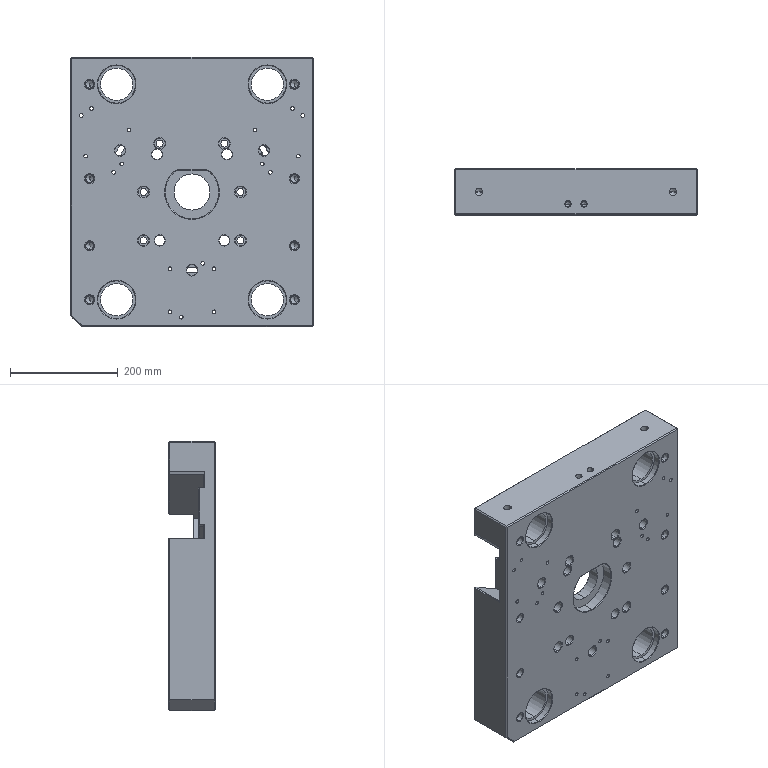Part | STEP file | P2 - 1 cav | 1 solid | 450 faces | box 450 x 86 x 500 mm | volume 13008282 mm3 | cylinder 164 | plane 153 | cone 133 | commonest cylinder face diameters 6.8 x36 14 x24 20 x20 17 x16 4 x14 10 x14